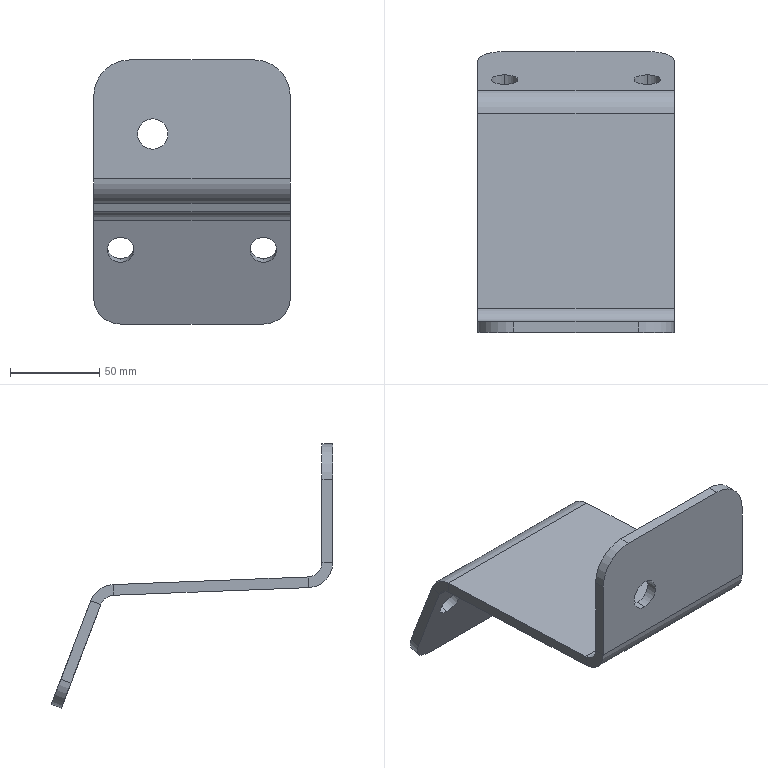Part | SolidWorks | features Fillet 2, ICE 2, FlatPattern 1, SMBaseFlange 1, SheetMetal 1 | 1 solid | 32 faces | box 110 x 157.607 x 148 mm | volume 171596 mm3 | plane 18 | cylinder 14 | commonest cylinder face diameters 15 x4 16 x2 17 x2 28 x2 30 x2 40 x2
STEP:
#1=CARTESIAN_POINT('',(-40.,133.488,-99.407));
#2=VERTEX_POINT('',#1);
#3=CARTESIAN_POINT('',(-40.,138.828,-113.424));
#4=VERTEX_POINT('',#3);
#5=CARTESIAN_POINT('',(-40.,136.158,-106.415));
#6=DIRECTION('',(0.,-0.9345,-0.356));
#7=DIRECTION('',(0.,-0.356,0.9345));
#8=AXIS2_PLACEMENT_3D('',#5,#6,#7);
#9=CIRCLE('',#8,7.5);
#10=EDGE_CURVE('',#2,#4,#9,.T.);
#11=ORIENTED_EDGE('',*,*,#10,.T.);
#12=CARTESIAN_POINT('',(-40.,144.435,-111.288));
#13=VERTEX_POINT('',#12);
#14=CARTESIAN_POINT('',(-40.,6.09,-163.991));
#15=DIRECTION('',(0.,0.9345,0.356));
#16=VECTOR('',#15,1000.);
#17=LINE('',#14,#16);
#18=EDGE_CURVE('',#4,#13,#17,.T.);
#19=ORIENTED_EDGE('',*,*,#18,.T.);
#20=CARTESIAN_POINT('',(-40.,139.095,-97.271));
#21=VERTEX_POINT('',#20);
#22=CARTESIAN_POINT('',(-40.,141.765,-104.279));
#23=DIRECTION('',(0.,0.9345,0.356));
#24=DIRECTION('',(0.,-0.356,0.9345));
#25=AXIS2_PLACEMENT_3D('',#22,#23,#24);
#26=CIRCLE('',#25,7.5);
#27=EDGE_CURVE('',#13,#21,#26,.T.);
#28=ORIENTED_EDGE('',*,*,#27,.T.);
#29=CARTESIAN_POINT('',(-40.,0.7504,-149.973));
#30=DIRECTION('',(0.,0.9345,0.356));
#31=VECTOR('',#30,1000.);
#32=LINE('',#29,#31);
#33=EDGE_CURVE('',#2,#21,#32,.T.);
#34=ORIENTED_EDGE('',*,*,#33,.F.);
#35=EDGE_LOOP('',(#11,#19,#28,#34));
#36=FACE_OUTER_BOUND('',#35,.T.);
#37=CARTESIAN_POINT('',(-40.,3.42,-156.982));
#38=DIRECTION('',(0.,0.9345,0.356));
#39=DIRECTION('',(0.,-0.356,0.9345));
#40=AXIS2_PLACEMENT_3D('',#37,#38,#39);
#41=CYLINDRICAL_SURFACE('',#40,7.5);
#42=ADVANCED_FACE('',(#36),#41,.F.);
#43=CARTESIAN_POINT('',(40.,133.488,-99.407));
#44=VERTEX_POINT('',#43);
#45=CARTESIAN_POINT('',(40.,138.828,-113.424));
#46=VERTEX_POINT('',#45);
#47=CARTESIAN_POINT('',(40.,136.158,-106.415));
#48=DIRECTION('',(0.,-0.9345,-0.356));
#49=DIRECTION('',(0.,-0.356,0.9345));
#50=AXIS2_PLACEMENT_3D('',#47,#48,#49);
#51=CIRCLE('',#50,7.5);
#52=EDGE_CURVE('',#44,#46,#51,.T.);
#53=ORIENTED_EDGE('',*,*,#52,.T.);
#54=CARTESIAN_POINT('',(40.,144.435,-111.288));
#55=VERTEX_POINT('',#54);
#56=CARTESIAN_POINT('',(40.,6.09,-163.991));
#57=DIRECTION('',(0.,0.9345,0.356));
#58=VECTOR('',#57,1000.);
#59=LINE('',#56,#58);
#60=EDGE_CURVE('',#46,#55,#59,.T.);
#61=ORIENTED_EDGE('',*,*,#60,.T.);
#62=CARTESIAN_POINT('',(40.,139.095,-97.271));
#63=VERTEX_POINT('',#62);
#64=CARTESIAN_POINT('',(40.,141.765,-104.279));
#65=DIRECTION('',(0.,0.9345,0.356));
#66=DIRECTION('',(0.,-0.356,0.9345));
#67=AXIS2_PLACEMENT_3D('',#64,#65,#66);
#68=CIRCLE('',#67,7.5);
#69=EDGE_CURVE('',#55,#63,#68,.T.);
#70=ORIENTED_EDGE('',*,*,#69,.T.);
#71=CARTESIAN_POINT('',(40.,0.7504,-149.973));
#72=DIRECTION('',(0.,0.9345,0.356));
#73=VECTOR('',#72,1000.);
#74=LINE('',#71,#73);
#75=EDGE_CURVE('',#44,#63,#74,.T.);
#76=ORIENTED_EDGE('',*,*,#75,.F.);
#77=EDGE_LOOP('',(#53,#61,#70,#76));
#78=FACE_OUTER_BOUND('',#77,.T.);
#79=CARTESIAN_POINT('',(40.,3.42,-156.982));
#80=DIRECTION('',(0.,0.9345,0.356));
#81=DIRECTION('',(0.,-0.356,0.9345));
#82=AXIS2_PLACEMENT_3D('',#79,#80,#81);
#83=CYLINDRICAL_SURFACE('',#82,7.5);
#84=ADVANCED_FACE('',(#78),#83,.F.);
#85=CARTESIAN_POINT('',(-22.,0.,-33.));
#86=VERTEX_POINT('',#85);
#87=CARTESIAN_POINT('',(-22.,0.,-50.));
#88=VERTEX_POINT('',#87);
#89=CARTESIAN_POINT('',(-22.,0.,-41.5));
#90=DIRECTION('',(0.,-1.,0.));
#91=DIRECTION('',(0.,0.,1.));
#92=AXIS2_PLACEMENT_3D('',#89,#90,#91);
#93=CIRCLE('',#92,8.5);
#94=EDGE_CURVE('',#86,#88,#93,.T.);
#95=ORIENTED_EDGE('',*,*,#94,.T.);
#96=CARTESIAN_POINT('',(-22.,6.,-50.));
#97=VERTEX_POINT('',#96);
#98=CARTESIAN_POINT('',(-22.,-0.001,-50.));
#99=DIRECTION('',(0.,1.,0.));
#100=VECTOR('',#99,1000.);
#101=LINE('',#98,#100);
#102=EDGE_CURVE('',#88,#97,#101,.T.);
#103=ORIENTED_EDGE('',*,*,#102,.T.);
#104=CARTESIAN_POINT('',(-22.,6.,-33.));
#105=VERTEX_POINT('',#104);
#106=CARTESIAN_POINT('',(-22.,6.,-41.5));
#107=DIRECTION('',(0.,1.,0.));
#108=DIRECTION('',(0.,0.,1.));
#109=AXIS2_PLACEMENT_3D('',#106,#107,#108);
#110=CIRCLE('',#109,8.5);
#111=EDGE_CURVE('',#97,#105,#110,.T.);
#112=ORIENTED_EDGE('',*,*,#111,.T.);
#113=CARTESIAN_POINT('',(-22.,-0.001,-33.));
#114=DIRECTION('',(0.,1.,0.));
#115=VECTOR('',#114,1000.);
#116=LINE('',#113,#115);
#117=EDGE_CURVE('',#86,#105,#116,.T.);
#118=ORIENTED_EDGE('',*,*,#117,.F.);
#119=EDGE_LOOP('',(#95,#103,#112,#118));
#120=FACE_OUTER_BOUND('',#119,.T.);
#121=CARTESIAN_POINT('',(-22.,-0.001,-41.5));
#122=DIRECTION('',(0.,1.,0.));
#123=DIRECTION('',(0.,0.,1.));
#124=AXIS2_PLACEMENT_3D('',#121,#122,#123);
#125=CYLINDRICAL_SURFACE('',#124,8.5);
#126=ADVANCED_FACE('',(#120),#125,.F.);
#127=CARTESIAN_POINT('',(55.,0.,-66.536));
#128=VERTEX_POINT('',#127);
#129=CARTESIAN_POINT('',(55.,6.,-66.536));
#130=VERTEX_POINT('',#129);
#131=CARTESIAN_POINT('',(55.,0.,-66.536));
#132=DIRECTION('',(0.,1.,0.));
#133=VECTOR('',#132,1000.);
#134=LINE('',#131,#133);
#135=EDGE_CURVE('',#128,#130,#134,.T.);
#136=ORIENTED_EDGE('',*,*,#135,.F.);
#137=CARTESIAN_POINT('',(55.,13.454,-80.526));
#138=VERTEX_POINT('',#137);
#139=CARTESIAN_POINT('',(55.,14.,-66.536));
#140=DIRECTION('',(1.,0.,0.));
#141=DIRECTION('',(0.,0.,1.));
#142=AXIS2_PLACEMENT_3D('',#139,#140,#141);
#143=CIRCLE('',#142,14.);
#144=EDGE_CURVE('',#128,#138,#143,.T.);
#145=ORIENTED_EDGE('',*,*,#144,.T.);
#146=CARTESIAN_POINT('',(55.,13.688,-74.53));
#147=VERTEX_POINT('',#146);
#148=CARTESIAN_POINT('',(55.,13.688,-74.53));
#149=DIRECTION('',(0.,-0.03903,-0.9992));
#150=VECTOR('',#149,1000.);
#151=LINE('',#148,#150);
#152=EDGE_CURVE('',#147,#138,#151,.T.);
#153=ORIENTED_EDGE('',*,*,#152,.F.);
#154=CARTESIAN_POINT('',(55.,14.,-66.536));
#155=DIRECTION('',(1.,0.,0.));
#156=DIRECTION('',(0.,0.,-1.));
#157=AXIS2_PLACEMENT_3D('',#154,#155,#156);
#158=CIRCLE('',#157,8.);
#159=EDGE_CURVE('',#130,#147,#158,.T.);
#160=ORIENTED_EDGE('',*,*,#159,.F.);
#161=EDGE_LOOP('',(#136,#145,#153,#160));
#162=FACE_OUTER_BOUND('',#161,.T.);
#163=CARTESIAN_POINT('',(55.,0.,-66.536));
#164=DIRECTION('',(1.,0.,0.));
#165=DIRECTION('',(0.,0.,-1.));
#166=AXIS2_PLACEMENT_3D('',#163,#164,#165);
#167=PLANE('',#166);
#168=ADVANCED_FACE('',(#162),#167,.T.);
#169=CARTESIAN_POINT('',(55.,6.,-20.));
#170=VERTEX_POINT('',#169);
#171=CARTESIAN_POINT('',(55.,6.,0.));
#172=DIRECTION('',(0.,0.,-1.));
#173=VECTOR('',#172,1000.);
#174=LINE('',#171,#173);
#175=EDGE_CURVE('',#170,#130,#174,.T.);
#176=ORIENTED_EDGE('',*,*,#175,.F.);
#177=CARTESIAN_POINT('',(55.,0.,-20.));
#178=VERTEX_POINT('',#177);
#179=CARTESIAN_POINT('',(55.,13.688,-20.));
#180=DIRECTION('',(0.,-1.,0.));
#181=VECTOR('',#180,1000.);
#182=LINE('',#179,#181);
#183=EDGE_CURVE('',#170,#178,#182,.T.);
#184=ORIENTED_EDGE('',*,*,#183,.T.);
#185=CARTESIAN_POINT('',(55.,0.,0.));
#186=DIRECTION('',(0.,0.,-1.));
#187=VECTOR('',#186,1000.);
#188=LINE('',#185,#187);
#189=EDGE_CURVE('',#178,#128,#188,.T.);
#190=ORIENTED_EDGE('',*,*,#189,.T.);
#191=ORIENTED_EDGE('',*,*,#135,.T.);
#192=EDGE_LOOP('',(#176,#184,#190,#191));
#193=FACE_OUTER_BOUND('',#192,.T.);
#194=CARTESIAN_POINT('',(55.,13.688,-74.53));
#195=DIRECTION('',(1.,0.,0.));
#196=DIRECTION('',(0.,0.,-1.));
#197=AXIS2_PLACEMENT_3D('',#194,#195,#196);
#198=PLANE('',#197);
#199=ADVANCED_FACE('',(#193),#198,.T.);
#200=CARTESIAN_POINT('',(-55.,13.454,-80.526));
#201=VERTEX_POINT('',#200);
#202=CARTESIAN_POINT('',(-55.,13.688,-74.53));
#203=VERTEX_POINT('',#202);
#204=CARTESIAN_POINT('',(-55.,13.454,-80.526));
#205=DIRECTION('',(0.,0.03903,0.9992));
#206=VECTOR('',#205,1000.);
#207=LINE('',#204,#206);
#208=EDGE_CURVE('',#201,#203,#207,.T.);
#209=ORIENTED_EDGE('',*,*,#208,.F.);
#210=CARTESIAN_POINT('',(-55.,0.,-66.536));
#211=VERTEX_POINT('',#210);
#212=CARTESIAN_POINT('',(-55.,14.,-66.536));
#213=DIRECTION('',(1.,0.,0.));
#214=DIRECTION('',(0.,0.,1.));
#215=AXIS2_PLACEMENT_3D('',#212,#213,#214);
#216=CIRCLE('',#215,14.);
#217=EDGE_CURVE('',#211,#201,#216,.T.);
#218=ORIENTED_EDGE('',*,*,#217,.F.);
#219=CARTESIAN_POINT('',(-55.,6.,-66.536));
#220=VERTEX_POINT('',#219);
#221=CARTESIAN_POINT('',(-55.,6.,-66.536));
#222=DIRECTION('',(0.,-1.,0.));
#223=VECTOR('',#222,1000.);
#224=LINE('',#221,#223);
#225=EDGE_CURVE('',#220,#211,#224,.T.);
#226=ORIENTED_EDGE('',*,*,#225,.F.);
#227=CARTESIAN_POINT('',(-55.,14.,-66.536));
#228=DIRECTION('',(1.,0.,0.));
#229=DIRECTION('',(0.,0.,-1.));
#230=AXIS2_PLACEMENT_3D('',#227,#228,#229);
#231=CIRCLE('',#230,8.);
#232=EDGE_CURVE('',#220,#203,#231,.T.);
#233=ORIENTED_EDGE('',*,*,#232,.T.);
#234=EDGE_LOOP('',(#209,#218,#226,#233));
#235=FACE_OUTER_BOUND('',#234,.T.);
#236=CARTESIAN_POINT('',(-55.,13.454,-80.526));
#237=DIRECTION('',(-1.,0.,0.));
#238=DIRECTION('',(0.,0.,1.));
#239=AXIS2_PLACEMENT_3D('',#236,#237,#238);
#240=PLANE('',#239);
#241=ADVANCED_FACE('',(#235),#240,.T.);
#242=CARTESIAN_POINT('',(-55.,122.718,-84.794));
#243=VERTEX_POINT('',#242);
#244=CARTESIAN_POINT('',(-55.,0.,-80.));
#245=DIRECTION('',(0.,0.9992,-0.03903));
#246=VECTOR('',#245,1000.);
#247=LINE('',#244,#246);
#248=EDGE_CURVE('',#201,#243,#247,.T.);
#249=ORIENTED_EDGE('',*,*,#248,.F.);
#250=ORIENTED_EDGE('',*,*,#208,.T.);
#251=CARTESIAN_POINT('',(-55.,122.952,-78.798));
#252=VERTEX_POINT('',#251);
#253=CARTESIAN_POINT('',(-55.,0.2342,-74.005));
#254=DIRECTION('',(0.,0.9992,-0.03903));
#255=VECTOR('',#254,1000.);
#256=LINE('',#253,#255);
#257=EDGE_CURVE('',#203,#252,#256,.T.);
#258=ORIENTED_EDGE('',*,*,#257,.T.);
#259=CARTESIAN_POINT('',(-55.,122.952,-78.798));
#260=DIRECTION('',(0.,-0.03903,-0.9992));
#261=VECTOR('',#260,1000.);
#262=LINE('',#259,#261);
#263=EDGE_CURVE('',#252,#243,#262,.T.);
#264=ORIENTED_EDGE('',*,*,#263,.T.);
#265=EDGE_LOOP('',(#249,#250,#258,#264));
#266=FACE_OUTER_BOUND('',#265,.T.);
#267=CARTESIAN_POINT('',(-55.,6.,-66.536));
#268=DIRECTION('',(-1.,0.,0.));
#269=DIRECTION('',(0.,0.,1.));
#270=AXIS2_PLACEMENT_3D('',#267,#268,#269);
#271=PLANE('',#270);
#272=ADVANCED_FACE('',(#266),#271,.T.);
#273=CARTESIAN_POINT('',(55.,122.718,-84.794));
#274=VERTEX_POINT('',#273);
#275=CARTESIAN_POINT('',(55.,122.952,-78.798));
#276=VERTEX_POINT('',#275);
#277=CARTESIAN_POINT('',(55.,122.718,-84.794));
#278=DIRECTION('',(0.,0.03903,0.9992));
#279=VECTOR('',#278,1000.);
#280=LINE('',#277,#279);
#281=EDGE_CURVE('',#274,#276,#280,.T.);
#282=ORIENTED_EDGE('',*,*,#281,.F.);
#283=CARTESIAN_POINT('',(55.,129.882,-89.94));
#284=VERTEX_POINT('',#283);
#285=CARTESIAN_POINT('',(55.,122.406,-92.788));
#286=DIRECTION('',(-1.,0.,0.));
#287=DIRECTION('',(0.,0.,-1.));
#288=AXIS2_PLACEMENT_3D('',#285,#286,#287);
#289=CIRCLE('',#288,8.);
#290=EDGE_CURVE('',#274,#284,#289,.T.);
#291=ORIENTED_EDGE('',*,*,#290,.T.);
#292=CARTESIAN_POINT('',(55.,135.489,-87.804));
#293=VERTEX_POINT('',#292);
#294=CARTESIAN_POINT('',(55.,135.489,-87.804));
#295=DIRECTION('',(0.,-0.9345,-0.356));
#296=VECTOR('',#295,1000.);
#297=LINE('',#294,#296);
#298=EDGE_CURVE('',#293,#284,#297,.T.);
#299=ORIENTED_EDGE('',*,*,#298,.F.);
#300=CARTESIAN_POINT('',(55.,122.406,-92.788));
#301=DIRECTION('',(-1.,0.,0.));
#302=DIRECTION('',(0.,0.,-1.));
#303=AXIS2_PLACEMENT_3D('',#300,#301,#302);
#304=CIRCLE('',#303,14.);
#305=EDGE_CURVE('',#276,#293,#304,.T.);
#306=ORIENTED_EDGE('',*,*,#305,.F.);
#307=EDGE_LOOP('',(#282,#291,#299,#306));
#308=FACE_OUTER_BOUND('',#307,.T.);
#309=CARTESIAN_POINT('',(55.,122.718,-84.794));
#310=DIRECTION('',(1.,0.,0.));
#311=DIRECTION('',(0.,0.,-1.));
#312=AXIS2_PLACEMENT_3D('',#309,#310,#311);
#313=PLANE('',#312);
#314=ADVANCED_FACE('',(#308),#313,.T.);
#315=CARTESIAN_POINT('',(55.,0.,-80.));
#316=DIRECTION('',(0.,0.9992,-0.03903));
#317=VECTOR('',#316,1000.);
#318=LINE('',#315,#317);
#319=EDGE_CURVE('',#138,#274,#318,.T.);
#320=ORIENTED_EDGE('',*,*,#319,.T.);
#321=ORIENTED_EDGE('',*,*,#281,.T.);
#322=CARTESIAN_POINT('',(55.,0.2342,-74.005));
#323=DIRECTION('',(0.,0.9992,-0.03903));
#324=VECTOR('',#323,1000.);
#325=LINE('',#322,#324);
#326=EDGE_CURVE('',#147,#276,#325,.T.);
#327=ORIENTED_EDGE('',*,*,#326,.F.);
#328=ORIENTED_EDGE('',*,*,#152,.T.);
#329=EDGE_LOOP('',(#320,#321,#327,#328));
#330=FACE_OUTER_BOUND('',#329,.T.);
#331=CARTESIAN_POINT('',(55.,135.489,-87.804));
#332=DIRECTION('',(1.,0.,0.));
#333=DIRECTION('',(0.,0.,-1.));
#334=AXIS2_PLACEMENT_3D('',#331,#332,#333);
#335=PLANE('',#334);
#336=ADVANCED_FACE('',(#330),#335,.T.);
#337=CARTESIAN_POINT('',(-55.,129.882,-89.94));
#338=VERTEX_POINT('',#337);
#339=CARTESIAN_POINT('',(-55.,135.489,-87.804));
#340=VERTEX_POINT('',#339);
#341=CARTESIAN_POINT('',(-55.,129.882,-89.94));
#342=DIRECTION('',(0.,0.9345,0.356));
#343=VECTOR('',#342,1000.);
#344=LINE('',#341,#343);
#345=EDGE_CURVE('',#338,#340,#344,.T.);
#346=ORIENTED_EDGE('',*,*,#345,.F.);
#347=CARTESIAN_POINT('',(-55.,122.406,-92.788));
#348=DIRECTION('',(-1.,0.,0.));
#349=DIRECTION('',(0.,0.,-1.));
#350=AXIS2_PLACEMENT_3D('',#347,#348,#349);
#351=CIRCLE('',#350,8.);
#352=EDGE_CURVE('',#243,#338,#351,.T.);
#353=ORIENTED_EDGE('',*,*,#352,.F.);
#354=ORIENTED_EDGE('',*,*,#263,.F.);
#355=CARTESIAN_POINT('',(-55.,122.406,-92.788));
#356=DIRECTION('',(-1.,0.,0.));
#357=DIRECTION('',(0.,0.,-1.));
#358=AXIS2_PLACEMENT_3D('',#355,#356,#357);
#359=CIRCLE('',#358,14.);
#360=EDGE_CURVE('',#252,#340,#359,.T.);
#361=ORIENTED_EDGE('',*,*,#360,.T.);
#362=EDGE_LOOP('',(#346,#353,#354,#361));
#363=FACE_OUTER_BOUND('',#362,.T.);
#364=CARTESIAN_POINT('',(-55.,129.882,-89.94));
#365=DIRECTION('',(-1.,0.,0.));
#366=DIRECTION('',(0.,0.,1.));
#367=AXIS2_PLACEMENT_3D('',#364,#365,#366);
#368=PLANE('',#367);
#369=ADVANCED_FACE('',(#363),#368,.T.);
#370=CARTESIAN_POINT('',(-55.,152.267,-131.847));
#371=VERTEX_POINT('',#370);
#372=CARTESIAN_POINT('',(-55.,133.607,-82.864));
#373=DIRECTION('',(0.,0.356,-0.9345));
#374=VECTOR('',#373,1000.);
#375=LINE('',#372,#374);
#376=EDGE_CURVE('',#340,#371,#375,.T.);
#377=ORIENTED_EDGE('',*,*,#376,.T.);
#378=CARTESIAN_POINT('',(-55.,146.66,-133.983));
#379=VERTEX_POINT('',#378);
#380=CARTESIAN_POINT('',(-55.,144.315,-134.876));
#381=DIRECTION('',(0.,-0.9345,-0.356));
#382=VECTOR('',#381,1000.);
#383=LINE('',#380,#382);
#384=EDGE_CURVE('',#371,#379,#383,.T.);
#385=ORIENTED_EDGE('',*,*,#384,.T.);
#386=CARTESIAN_POINT('',(-55.,128.,-85.));
#387=DIRECTION('',(0.,0.356,-0.9345));
#388=VECTOR('',#387,1000.);
#389=LINE('',#386,#388);
#390=EDGE_CURVE('',#338,#379,#389,.T.);
#391=ORIENTED_EDGE('',*,*,#390,.F.);
#392=ORIENTED_EDGE('',*,*,#345,.T.);
#393=EDGE_LOOP('',(#377,#385,#391,#392));
#394=FACE_OUTER_BOUND('',#393,.T.);
#395=CARTESIAN_POINT('',(-55.,122.952,-78.798));
#396=DIRECTION('',(-1.,0.,0.));
#397=DIRECTION('',(0.,0.,1.));
#398=AXIS2_PLACEMENT_3D('',#395,#396,#397);
#399=PLANE('',#398);
#400=ADVANCED_FACE('',(#394),#399,.T.);
#401=ORIENTED_EDGE('',*,*,#10,.F.);
#402=CARTESIAN_POINT('',(-40.,136.158,-106.415));
#403=DIRECTION('',(0.,-0.9345,-0.356));
#404=DIRECTION('',(0.,-0.356,0.9345));
#405=AXIS2_PLACEMENT_3D('',#402,#403,#404);
#406=CIRCLE('',#405,7.5);
#407=EDGE_CURVE('',#4,#2,#406,.T.);
#408=ORIENTED_EDGE('',*,*,#407,.F.);
#409=EDGE_LOOP('',(#401,#408));
#410=FACE_BOUND('',#409,.T.);
#411=ORIENTED_EDGE('',*,*,#52,.F.);
#412=CARTESIAN_POINT('',(40.,136.158,-106.415));
#413=DIRECTION('',(0.,-0.9345,-0.356));
#414=DIRECTION('',(0.,-0.356,0.9345));
#415=AXIS2_PLACEMENT_3D('',#412,#413,#414);
#416=CIRCLE('',#415,7.5);
#417=EDGE_CURVE('',#46,#44,#416,.T.);
#418=ORIENTED_EDGE('',*,*,#417,.F.);
#419=EDGE_LOOP('',(#411,#418));
#420=FACE_BOUND('',#419,.T.);
#421=ORIENTED_EDGE('',*,*,#390,.T.);
#422=CARTESIAN_POINT('',(-40.,152.,-148.));
#423=VERTEX_POINT('',#422);
#424=CARTESIAN_POINT('',(-40.,146.66,-133.983));
#425=DIRECTION('',(0.,-0.9345,-0.356));
#426=DIRECTION('',(0.,-0.356,0.9345));
#427=AXIS2_PLACEMENT_3D('',#424,#425,#426);
#428=CIRCLE('',#427,15.);
#429=EDGE_CURVE('',#379,#423,#428,.T.);
#430=ORIENTED_EDGE('',*,*,#429,.T.);
#431=CARTESIAN_POINT('',(40.,152.,-148.));
#432=VERTEX_POINT('',#431);
#433=CARTESIAN_POINT('',(55.,152.,-148.));
#434=DIRECTION('',(-1.,0.,0.));
#435=VECTOR('',#434,1000.);
#436=LINE('',#433,#435);
#437=EDGE_CURVE('',#432,#423,#436,.T.);
#438=ORIENTED_EDGE('',*,*,#437,.F.);
#439=CARTESIAN_POINT('',(55.,146.66,-133.983));
#440=VERTEX_POINT('',#439);
#441=CARTESIAN_POINT('',(40.,146.66,-133.983));
#442=DIRECTION('',(0.,-0.9345,-0.356));
#443=DIRECTION('',(0.,-0.356,0.9345));
#444=AXIS2_PLACEMENT_3D('',#441,#442,#443);
#445=CIRCLE('',#444,15.);
#446=EDGE_CURVE('',#432,#440,#445,.T.);
#447=ORIENTED_EDGE('',*,*,#446,.T.);
#448=CARTESIAN_POINT('',(55.,128.,-85.));
#449=DIRECTION('',(0.,0.356,-0.9345));
#450=VECTOR('',#449,1000.);
#451=LINE('',#448,#450);
#452=EDGE_CURVE('',#284,#440,#451,.T.);
#453=ORIENTED_EDGE('',*,*,#452,.F.);
#454=CARTESIAN_POINT('',(55.,129.882,-89.94));
#455=DIRECTION('',(-1.,0.,0.));
#456=VECTOR('',#455,1000.);
#457=LINE('',#454,#456);
#458=EDGE_CURVE('',#284,#338,#457,.T.);
#459=ORIENTED_EDGE('',*,*,#458,.T.);
#460=EDGE_LOOP('',(#421,#430,#438,#447,#453,#459));
#461=FACE_OUTER_BOUND('',#460,.T.);
#462=CARTESIAN_POINT('',(55.,128.,-85.));
#463=DIRECTION('',(0.,0.9345,0.356));
#464=DIRECTION('',(0.,-0.356,0.9345));
#465=AXIS2_PLACEMENT_3D('',#462,#463,#464);
#466=PLANE('',#465);
#467=ADVANCED_FACE('',(#410,#420,#461),#466,.F.);
#468=ORIENTED_EDGE('',*,*,#437,.T.);
#469=CARTESIAN_POINT('',(-40.,157.607,-145.864));
#470=VERTEX_POINT('',#469);
#471=CARTESIAN_POINT('',(-40.,157.607,-145.864));
#472=DIRECTION('',(0.,0.9345,0.356));
#473=VECTOR('',#472,1000.);
#474=LINE('',#471,#473);
#475=EDGE_CURVE('',#423,#470,#474,.T.);
#476=ORIENTED_EDGE('',*,*,#475,.T.);
#477=CARTESIAN_POINT('',(40.,157.607,-145.864));
#478=VERTEX_POINT('',#477);
#479=CARTESIAN_POINT('',(55.,157.607,-145.864));
#480=DIRECTION('',(-1.,0.,0.));
#481=VECTOR('',#480,1000.);
#482=LINE('',#479,#481);
#483=EDGE_CURVE('',#478,#470,#482,.T.);
#484=ORIENTED_EDGE('',*,*,#483,.F.);
#485=CARTESIAN_POINT('',(40.,157.607,-145.864));
#486=DIRECTION('',(0.,-0.9345,-0.356));
#487=VECTOR('',#486,1000.);
#488=LINE('',#485,#487);
#489=EDGE_CURVE('',#478,#432,#488,.T.);
#490=ORIENTED_EDGE('',*,*,#489,.T.);
#491=EDGE_LOOP('',(#468,#476,#484,#490));
#492=FACE_OUTER_BOUND('',#491,.T.);
#493=CARTESIAN_POINT('',(55.,157.607,-145.864));
#494=DIRECTION('',(0.,0.356,-0.9345));
#495=DIRECTION('',(0.,0.9345,0.356));
#496=AXIS2_PLACEMENT_3D('',#493,#494,#495);
#497=PLANE('',#496);
#498=ADVANCED_FACE('',(#492),#497,.T.);
#499=CARTESIAN_POINT('',(-40.,141.765,-104.279));
#500=DIRECTION('',(0.,0.9345,0.356));
#501=DIRECTION('',(0.,-0.356,0.9345));
#502=AXIS2_PLACEMENT_3D('',#499,#500,#501);
#503=CIRCLE('',#502,7.5);
#504=EDGE_CURVE('',#21,#13,#503,.T.);
#505=ORIENTED_EDGE('',*,*,#504,.F.);
#506=ORIENTED_EDGE('',*,*,#27,.F.);
#507=EDGE_LOOP('',(#505,#506));
#508=FACE_BOUND('',#507,.T.);
#509=CARTESIAN_POINT('',(40.,141.765,-104.279));
#510=DIRECTION('',(0.,0.9345,0.356));
#511=DIRECTION('',(0.,-0.356,0.9345));
#512=AXIS2_PLACEMENT_3D('',#509,#510,#511);
#513=CIRCLE('',#512,7.5);
#514=EDGE_CURVE('',#63,#55,#513,.T.);
#515=ORIENTED_EDGE('',*,*,#514,.F.);
#516=ORIENTED_EDGE('',*,*,#69,.F.);
#517=EDGE_LOOP('',(#515,#516));
#518=FACE_BOUND('',#517,.T.);
#519=ORIENTED_EDGE('',*,*,#483,.T.);
#520=CARTESIAN_POINT('',(-40.,152.267,-131.847));
#521=DIRECTION('',(0.,0.9345,0.356));
#522=DIRECTION('',(0.,-0.356,0.9345));
#523=AXIS2_PLACEMENT_3D('',#520,#521,#522);
#524=CIRCLE('',#523,15.);
#525=EDGE_CURVE('',#470,#371,#524,.T.);
#526=ORIENTED_EDGE('',*,*,#525,.T.);
#527=ORIENTED_EDGE('',*,*,#376,.F.);
#528=CARTESIAN_POINT('',(55.,135.489,-87.804));
#529=DIRECTION('',(-1.,0.,0.));
#530=VECTOR('',#529,1000.);
#531=LINE('',#528,#530);
#532=EDGE_CURVE('',#293,#340,#531,.T.);
#533=ORIENTED_EDGE('',*,*,#532,.F.);
#534=CARTESIAN_POINT('',(55.,152.267,-131.847));
#535=VERTEX_POINT('',#534);
#536=CARTESIAN_POINT('',(55.,133.607,-82.864));
#537=DIRECTION('',(0.,0.356,-0.9345));
#538=VECTOR('',#537,1000.);
#539=LINE('',#536,#538);
#540=EDGE_CURVE('',#293,#535,#539,.T.);
#541=ORIENTED_EDGE('',*,*,#540,.T.);
#542=CARTESIAN_POINT('',(40.,152.267,-131.847));
#543=DIRECTION('',(0.,0.9345,0.356));
#544=DIRECTION('',(0.,-0.356,0.9345));
#545=AXIS2_PLACEMENT_3D('',#542,#543,#544);
#546=CIRCLE('',#545,15.);
#547=EDGE_CURVE('',#535,#478,#546,.T.);
#548=ORIENTED_EDGE('',*,*,#547,.T.);
#549=EDGE_LOOP('',(#519,#526,#527,#533,#541,#548));
#550=FACE_OUTER_BOUND('',#549,.T.);
#551=CARTESIAN_POINT('',(55.,133.607,-82.864));
#552=DIRECTION('',(0.,0.9345,0.356));
#553=DIRECTION('',(0.,-0.356,0.9345));
#554=AXIS2_PLACEMENT_3D('',#551,#552,#553);
#555=PLANE('',#554);
#556=ADVANCED_FACE('',(#508,#518,#550),#555,.T.);
#557=ORIENTED_EDGE('',*,*,#360,.F.);
#558=CARTESIAN_POINT('',(55.,122.952,-78.798));
#559=DIRECTION('',(-1.,0.,0.));
#560=VECTOR('',#559,1000.);
#561=LINE('',#558,#560);
#562=EDGE_CURVE('',#276,#252,#561,.T.);
#563=ORIENTED_EDGE('',*,*,#562,.F.);
#564=ORIENTED_EDGE('',*,*,#305,.T.);
#565=ORIENTED_EDGE('',*,*,#532,.T.);
#566=EDGE_LOOP('',(#557,#563,#564,#565));
#567=FACE_OUTER_BOUND('',#566,.T.);
#568=CARTESIAN_POINT('',(55.,122.406,-92.788));
#569=DIRECTION('',(-1.,0.,0.));
#570=DIRECTION('',(0.,0.,1.));
#571=AXIS2_PLACEMENT_3D('',#568,#569,#570);
#572=CYLINDRICAL_SURFACE('',#571,14.);
#573=ADVANCED_FACE('',(#567),#572,.T.);
#574=ORIENTED_EDGE('',*,*,#257,.F.);
#575=CARTESIAN_POINT('',(55.,13.688,-74.53));
#576=DIRECTION('',(-1.,0.,0.));
#577=VECTOR('',#576,1000.);
#578=LINE('',#575,#577);
#579=EDGE_CURVE('',#147,#203,#578,.T.);
#580=ORIENTED_EDGE('',*,*,#579,.F.);
#581=ORIENTED_EDGE('',*,*,#326,.T.);
#582=ORIENTED_EDGE('',*,*,#562,.T.);
#583=EDGE_LOOP('',(#574,#580,#581,#582));
#584=FACE_OUTER_BOUND('',#583,.T.);
#585=CARTESIAN_POINT('',(55.,0.2342,-74.005));
#586=DIRECTION('',(0.,0.03903,0.9992));
#587=DIRECTION('',(0.,-0.9992,0.03903));
#588=AXIS2_PLACEMENT_3D('',#585,#586,#587);
#589=PLANE('',#588);
#590=ADVANCED_FACE('',(#584),#589,.T.);
#591=ORIENTED_EDGE('',*,*,#232,.F.);
#592=CARTESIAN_POINT('',(55.,6.,-66.536));
#593=DIRECTION('',(-1.,0.,0.));
#594=VECTOR('',#593,1000.);
#595=LINE('',#592,#594);
#596=EDGE_CURVE('',#130,#220,#595,.T.);
#597=ORIENTED_EDGE('',*,*,#596,.F.);
#598=ORIENTED_EDGE('',*,*,#159,.T.);
#599=ORIENTED_EDGE('',*,*,#579,.T.);
#600=EDGE_LOOP('',(#591,#597,#598,#599));
#601=FACE_OUTER_BOUND('',#600,.T.);
#602=CARTESIAN_POINT('',(55.,14.,-66.536));
#603=DIRECTION('',(-1.,0.,0.));
#604=DIRECTION('',(0.,0.,1.));
#605=AXIS2_PLACEMENT_3D('',#602,#603,#604);
#606=CYLINDRICAL_SURFACE('',#605,8.);
#607=ADVANCED_FACE('',(#601),#606,.F.);
#608=CARTESIAN_POINT('',(-22.,6.,-41.5));
#609=DIRECTION('',(0.,1.,0.));
#610=DIRECTION('',(0.,0.,1.));
#611=AXIS2_PLACEMENT_3D('',#608,#609,#610);
#612=CIRCLE('',#611,8.5);
#613=EDGE_CURVE('',#105,#97,#612,.T.);
#614=ORIENTED_EDGE('',*,*,#613,.F.);
#615=ORIENTED_EDGE('',*,*,#111,.F.);
#616=EDGE_LOOP('',(#614,#615));
#617=FACE_BOUND('',#616,.T.);
#618=CARTESIAN_POINT('',(35.,6.,0.));
#619=VERTEX_POINT('',#618);
#620=CARTESIAN_POINT('',(-35.,6.,0.));
#621=VERTEX_POINT('',#620);
#622=CARTESIAN_POINT('',(55.,6.,0.));
#623=DIRECTION('',(-1.,0.,0.));
#624=VECTOR('',#623,1000.);
#625=LINE('',#622,#624);
#626=EDGE_CURVE('',#619,#621,#625,.T.);
#627=ORIENTED_EDGE('',*,*,#626,.F.);
#628=CARTESIAN_POINT('',(35.,6.,-20.));
#629=DIRECTION('',(0.,1.,0.));
#630=DIRECTION('',(0.,0.,1.));
#631=AXIS2_PLACEMENT_3D('',#628,#629,#630);
#632=CIRCLE('',#631,20.);
#633=EDGE_CURVE('',#619,#170,#632,.T.);
#634=ORIENTED_EDGE('',*,*,#633,.T.);
#635=ORIENTED_EDGE('',*,*,#175,.T.);
#636=ORIENTED_EDGE('',*,*,#596,.T.);
#637=CARTESIAN_POINT('',(-55.,6.,-20.));
#638=VERTEX_POINT('',#637);
#639=CARTESIAN_POINT('',(-55.,6.,0.));
#640=DIRECTION('',(0.,0.,-1.));
#641=VECTOR('',#640,1000.);
#642=LINE('',#639,#641);
#643=EDGE_CURVE('',#638,#220,#642,.T.);
#644=ORIENTED_EDGE('',*,*,#643,.F.);
#645=CARTESIAN_POINT('',(-35.,6.,-20.));
#646=DIRECTION('',(0.,1.,0.));
#647=DIRECTION('',(0.,0.,1.));
#648=AXIS2_PLACEMENT_3D('',#645,#646,#647);
#649=CIRCLE('',#648,20.);
#650=EDGE_CURVE('',#638,#621,#649,.T.);
#651=ORIENTED_EDGE('',*,*,#650,.T.);
#652=EDGE_LOOP('',(#627,#634,#635,#636,#644,#651));
#653=FACE_OUTER_BOUND('',#652,.T.);
#654=CARTESIAN_POINT('',(55.,6.,0.));
#655=DIRECTION('',(0.,1.,0.));
#656=DIRECTION('',(0.,0.,1.));
#657=AXIS2_PLACEMENT_3D('',#654,#655,#656);
#658=PLANE('',#657);
#659=ADVANCED_FACE('',(#617,#653),#658,.T.);
#660=CARTESIAN_POINT('',(35.,0.,0.));
#661=VERTEX_POINT('',#660);
#662=CARTESIAN_POINT('',(-35.,0.,0.));
#663=VERTEX_POINT('',#662);
#664=CARTESIAN_POINT('',(55.,0.,0.));
#665=DIRECTION('',(-1.,0.,0.));
#666=VECTOR('',#665,1000.);
#667=LINE('',#664,#666);
#668=EDGE_CURVE('',#661,#663,#667,.T.);
#669=ORIENTED_EDGE('',*,*,#668,.F.);
#670=CARTESIAN_POINT('',(35.,0.,0.));
#671=DIRECTION('',(0.,1.,0.));
#672=VECTOR('',#671,1000.);
#673=LINE('',#670,#672);
#674=EDGE_CURVE('',#661,#619,#673,.T.);
#675=ORIENTED_EDGE('',*,*,#674,.T.);
#676=ORIENTED_EDGE('',*,*,#626,.T.);
#677=CARTESIAN_POINT('',(-35.,0.,0.));
#678=DIRECTION('',(0.,-1.,0.));
#679=VECTOR('',#678,1000.);
#680=LINE('',#677,#679);
#681=EDGE_CURVE('',#621,#663,#680,.T.);
#682=ORIENTED_EDGE('',*,*,#681,.T.);
#683=EDGE_LOOP('',(#669,#675,#676,#682));
#684=FACE_OUTER_BOUND('',#683,.T.);
#685=CARTESIAN_POINT('',(55.,0.,0.));
#686=DIRECTION('',(0.,0.,1.));
#687=DIRECTION('',(1.,0.,0.));
#688=AXIS2_PLACEMENT_3D('',#685,#686,#687);
#689=PLANE('',#688);
#690=ADVANCED_FACE('',(#684),#689,.T.);
#691=ORIENTED_EDGE('',*,*,#94,.F.);
#692=CARTESIAN_POINT('',(-22.,0.,-41.5));
#693=DIRECTION('',(0.,-1.,0.));
#694=DIRECTION('',(0.,0.,1.));
#695=AXIS2_PLACEMENT_3D('',#692,#693,#694);
#696=CIRCLE('',#695,8.5);
#697=EDGE_CURVE('',#88,#86,#696,.T.);
#698=ORIENTED_EDGE('',*,*,#697,.F.);
#699=EDGE_LOOP('',(#691,#698));
#700=FACE_BOUND('',#699,.T.);
#701=ORIENTED_EDGE('',*,*,#189,.F.);
#702=CARTESIAN_POINT('',(35.,0.,-20.));
#703=DIRECTION('',(0.,-1.,0.));
#704=DIRECTION('',(0.,0.,1.));
#705=AXIS2_PLACEMENT_3D('',#702,#703,#704);
#706=CIRCLE('',#705,20.);
#707=EDGE_CURVE('',#178,#661,#706,.T.);
#708=ORIENTED_EDGE('',*,*,#707,.T.);
#709=ORIENTED_EDGE('',*,*,#668,.T.);
#710=CARTESIAN_POINT('',(-55.,0.,-20.));
#711=VERTEX_POINT('',#710);
#712=CARTESIAN_POINT('',(-35.,0.,-20.));
#713=DIRECTION('',(0.,-1.,0.));
#714=DIRECTION('',(0.,0.,1.));
#715=AXIS2_PLACEMENT_3D('',#712,#713,#714);
#716=CIRCLE('',#715,20.);
#717=EDGE_CURVE('',#663,#711,#716,.T.);
#718=ORIENTED_EDGE('',*,*,#717,.T.);
#719=CARTESIAN_POINT('',(-55.,0.,0.));
#720=DIRECTION('',(0.,0.,-1.));
#721=VECTOR('',#720,1000.);
#722=LINE('',#719,#721);
#723=EDGE_CURVE('',#711,#211,#722,.T.);
#724=ORIENTED_EDGE('',*,*,#723,.T.);
#725=CARTESIAN_POINT('',(55.,0.,-66.536));
#726=DIRECTION('',(-1.,0.,0.));
#727=VECTOR('',#726,1000.);
#728=LINE('',#725,#727);
#729=EDGE_CURVE('',#128,#211,#728,.T.);
#730=ORIENTED_EDGE('',*,*,#729,.F.);
#731=EDGE_LOOP('',(#701,#708,#709,#718,#724,#730));
#732=FACE_OUTER_BOUND('',#731,.T.);
#733=CARTESIAN_POINT('',(55.,0.,0.));
#734=DIRECTION('',(0.,1.,0.));
#735=DIRECTION('',(0.,0.,1.));
#736=AXIS2_PLACEMENT_3D('',#733,#734,#735);
#737=PLANE('',#736);
#738=ADVANCED_FACE('',(#700,#732),#737,.F.);
#739=ORIENTED_EDGE('',*,*,#217,.T.);
#740=CARTESIAN_POINT('',(55.,13.454,-80.526));
#741=DIRECTION('',(-1.,0.,0.));
#742=VECTOR('',#741,1000.);
#743=LINE('',#740,#742);
#744=EDGE_CURVE('',#138,#201,#743,.T.);
#745=ORIENTED_EDGE('',*,*,#744,.F.);
#746=ORIENTED_EDGE('',*,*,#144,.F.);
#747=ORIENTED_EDGE('',*,*,#729,.T.);
#748=EDGE_LOOP('',(#739,#745,#746,#747));
#749=FACE_OUTER_BOUND('',#748,.T.);
#750=CARTESIAN_POINT('',(55.,14.,-66.536));
#751=DIRECTION('',(-1.,0.,0.));
#752=DIRECTION('',(0.,0.,1.));
#753=AXIS2_PLACEMENT_3D('',#750,#751,#752);
#754=CYLINDRICAL_SURFACE('',#753,14.);
#755=ADVANCED_FACE('',(#749),#754,.T.);
#756=ORIENTED_EDGE('',*,*,#248,.T.);
#757=CARTESIAN_POINT('',(55.,122.718,-84.794));
#758=DIRECTION('',(-1.,0.,0.));
#759=VECTOR('',#758,1000.);
#760=LINE('',#757,#759);
#761=EDGE_CURVE('',#274,#243,#760,.T.);
#762=ORIENTED_EDGE('',*,*,#761,.F.);
#763=ORIENTED_EDGE('',*,*,#319,.F.);
#764=ORIENTED_EDGE('',*,*,#744,.T.);
#765=EDGE_LOOP('',(#756,#762,#763,#764));
#766=FACE_OUTER_BOUND('',#765,.T.);
#767=CARTESIAN_POINT('',(55.,0.,-80.));
#768=DIRECTION('',(0.,0.03903,0.9992));
#769=DIRECTION('',(0.,-0.9992,0.03903));
#770=AXIS2_PLACEMENT_3D('',#767,#768,#769);
#771=PLANE('',#770);
#772=ADVANCED_FACE('',(#766),#771,.F.);
#773=ORIENTED_EDGE('',*,*,#352,.T.);
#774=ORIENTED_EDGE('',*,*,#458,.F.);
#775=ORIENTED_EDGE('',*,*,#290,.F.);
#776=ORIENTED_EDGE('',*,*,#761,.T.);
#777=EDGE_LOOP('',(#773,#774,#775,#776));
#778=FACE_OUTER_BOUND('',#777,.T.);
#779=CARTESIAN_POINT('',(55.,122.406,-92.788));
#780=DIRECTION('',(-1.,0.,0.));
#781=DIRECTION('',(0.,0.,1.));
#782=AXIS2_PLACEMENT_3D('',#779,#780,#781);
#783=CYLINDRICAL_SURFACE('',#782,8.);
#784=ADVANCED_FACE('',(#778),#783,.F.);
#785=ORIENTED_EDGE('',*,*,#452,.T.);
#786=CARTESIAN_POINT('',(55.,139.184,-136.831));
#787=DIRECTION('',(0.,0.9345,0.356));
#788=VECTOR('',#787,1000.);
#789=LINE('',#786,#788);
#790=EDGE_CURVE('',#440,#535,#789,.T.);
#791=ORIENTED_EDGE('',*,*,#790,.T.);
#792=ORIENTED_EDGE('',*,*,#540,.F.);
#793=ORIENTED_EDGE('',*,*,#298,.T.);
#794=EDGE_LOOP('',(#785,#791,#792,#793));
#795=FACE_OUTER_BOUND('',#794,.T.);
#796=CARTESIAN_POINT('',(55.,122.406,-92.788));
#797=DIRECTION('',(1.,0.,0.));
#798=DIRECTION('',(0.,0.,-1.));
#799=AXIS2_PLACEMENT_3D('',#796,#797,#798);
#800=PLANE('',#799);
#801=ADVANCED_FACE('',(#795),#800,.T.);
#802=ORIENTED_EDGE('',*,*,#723,.F.);
#803=CARTESIAN_POINT('',(-55.,6.,-20.));
#804=DIRECTION('',(0.,1.,0.));
#805=VECTOR('',#804,1000.);
#806=LINE('',#803,#805);
#807=EDGE_CURVE('',#711,#638,#806,.T.);
#808=ORIENTED_EDGE('',*,*,#807,.T.);
#809=ORIENTED_EDGE('',*,*,#643,.T.);
#810=ORIENTED_EDGE('',*,*,#225,.T.);
#811=EDGE_LOOP('',(#802,#808,#809,#810));
#812=FACE_OUTER_BOUND('',#811,.T.);
#813=CARTESIAN_POINT('',(-55.,122.406,-92.788));
#814=DIRECTION('',(1.,0.,0.));
#815=DIRECTION('',(0.,0.,-1.));
#816=AXIS2_PLACEMENT_3D('',#813,#814,#815);
#817=PLANE('',#816);
#818=ADVANCED_FACE('',(#812),#817,.F.);
#819=ORIENTED_EDGE('',*,*,#102,.F.);
#820=ORIENTED_EDGE('',*,*,#697,.T.);
#821=ORIENTED_EDGE('',*,*,#117,.T.);
#822=ORIENTED_EDGE('',*,*,#613,.T.);
#823=EDGE_LOOP('',(#819,#820,#821,#822));
#824=FACE_OUTER_BOUND('',#823,.T.);
#825=CARTESIAN_POINT('',(-22.,-0.001,-41.5));
#826=DIRECTION('',(0.,1.,0.));
#827=DIRECTION('',(0.,0.,1.));
#828=AXIS2_PLACEMENT_3D('',#825,#826,#827);
#829=CYLINDRICAL_SURFACE('',#828,8.5);
#830=ADVANCED_FACE('',(#824),#829,.F.);
#831=ORIENTED_EDGE('',*,*,#60,.F.);
#832=ORIENTED_EDGE('',*,*,#417,.T.);
#833=ORIENTED_EDGE('',*,*,#75,.T.);
#834=ORIENTED_EDGE('',*,*,#514,.T.);
#835=EDGE_LOOP('',(#831,#832,#833,#834));
#836=FACE_OUTER_BOUND('',#835,.T.);
#837=CARTESIAN_POINT('',(40.,3.42,-156.982));
#838=DIRECTION('',(0.,0.9345,0.356));
#839=DIRECTION('',(0.,-0.356,0.9345));
#840=AXIS2_PLACEMENT_3D('',#837,#838,#839);
#841=CYLINDRICAL_SURFACE('',#840,7.5);
#842=ADVANCED_FACE('',(#836),#841,.F.);
#843=ORIENTED_EDGE('',*,*,#18,.F.);
#844=ORIENTED_EDGE('',*,*,#407,.T.);
#845=ORIENTED_EDGE('',*,*,#33,.T.);
#846=ORIENTED_EDGE('',*,*,#504,.T.);
#847=EDGE_LOOP('',(#843,#844,#845,#846));
#848=FACE_OUTER_BOUND('',#847,.T.);
#849=CARTESIAN_POINT('',(-40.,3.42,-156.982));
#850=DIRECTION('',(0.,0.9345,0.356));
#851=DIRECTION('',(0.,-0.356,0.9345));
#852=AXIS2_PLACEMENT_3D('',#849,#850,#851);
#853=CYLINDRICAL_SURFACE('',#852,7.5);
#854=ADVANCED_FACE('',(#848),#853,.F.);
#855=ORIENTED_EDGE('',*,*,#707,.F.);
#856=ORIENTED_EDGE('',*,*,#183,.F.);
#857=ORIENTED_EDGE('',*,*,#633,.F.);
#858=ORIENTED_EDGE('',*,*,#674,.F.);
#859=EDGE_LOOP('',(#855,#856,#857,#858));
#860=FACE_OUTER_BOUND('',#859,.T.);
#861=CARTESIAN_POINT('',(35.,0.,-20.));
#862=DIRECTION('',(0.,1.,0.));
#863=DIRECTION('',(0.,0.,1.));
#864=AXIS2_PLACEMENT_3D('',#861,#862,#863);
#865=CYLINDRICAL_SURFACE('',#864,20.);
#866=ADVANCED_FACE('',(#860),#865,.T.);
#867=ORIENTED_EDGE('',*,*,#717,.F.);
#868=ORIENTED_EDGE('',*,*,#681,.F.);
#869=ORIENTED_EDGE('',*,*,#650,.F.);
#870=ORIENTED_EDGE('',*,*,#807,.F.);
#871=EDGE_LOOP('',(#867,#868,#869,#870));
#872=FACE_OUTER_BOUND('',#871,.T.);
#873=CARTESIAN_POINT('',(-35.,122.406,-20.));
#874=DIRECTION('',(0.,-1.,0.));
#875=DIRECTION('',(0.,0.,-1.));
#876=AXIS2_PLACEMENT_3D('',#873,#874,#875);
#877=CYLINDRICAL_SURFACE('',#876,20.);
#878=ADVANCED_FACE('',(#872),#877,.T.);
#879=ORIENTED_EDGE('',*,*,#525,.F.);
#880=ORIENTED_EDGE('',*,*,#475,.F.);
#881=ORIENTED_EDGE('',*,*,#429,.F.);
#882=ORIENTED_EDGE('',*,*,#384,.F.);
#883=EDGE_LOOP('',(#879,#880,#881,#882));
#884=FACE_OUTER_BOUND('',#883,.T.);
#885=CARTESIAN_POINT('',(-40.,144.315,-134.876));
#886=DIRECTION('',(0.,-0.9345,-0.356));
#887=DIRECTION('',(0.,0.356,-0.9345));
#888=AXIS2_PLACEMENT_3D('',#885,#886,#887);
#889=CYLINDRICAL_SURFACE('',#888,15.);
#890=ADVANCED_FACE('',(#884),#889,.T.);
#891=ORIENTED_EDGE('',*,*,#547,.F.);
#892=ORIENTED_EDGE('',*,*,#790,.F.);
#893=ORIENTED_EDGE('',*,*,#446,.F.);
#894=ORIENTED_EDGE('',*,*,#489,.F.);
#895=EDGE_LOOP('',(#891,#892,#893,#894));
#896=FACE_OUTER_BOUND('',#895,.T.);
#897=CARTESIAN_POINT('',(40.,152.267,-131.847));
#898=DIRECTION('',(0.,-0.9345,-0.356));
#899=DIRECTION('',(0.,0.356,-0.9345));
#900=AXIS2_PLACEMENT_3D('',#897,#898,#899);
#901=CYLINDRICAL_SURFACE('',#900,15.);
#902=ADVANCED_FACE('',(#896),#901,.T.);
#903=CLOSED_SHELL('',(#42,#84,#126,#168,#199,#241,#272,#314,#336,#369,#400,#467,#498,#556,#573,#590,#607,#659,#690,#738,#755,#772,#784,#801,#818,#830,#842,#854,#866,#878,#890,#902));
#904=MANIFOLD_SOLID_BREP('',#903);
#905=CARTESIAN_POINT('',(0.,0.,0.));
#906=DIRECTION('',(0.,0.,1.));
#907=DIRECTION('',(1.,0.,0.));
#908=AXIS2_PLACEMENT_3D('',#905,#906,#907);
#909=(LENGTH_UNIT()NAMED_UNIT(*)SI_UNIT(.MILLI.,.METRE.));
#910=UNCERTAINTY_MEASURE_WITH_UNIT(LENGTH_MEASURE(0.00001),#909,'','');
#911=(NAMED_UNIT(*)PLANE_ANGLE_UNIT()SI_UNIT($,.RADIAN.));
#912=(NAMED_UNIT(*)SI_UNIT($,.STERADIAN.)SOLID_ANGLE_UNIT());
#913=(GEOMETRIC_REPRESENTATION_CONTEXT(3)GLOBAL_UNCERTAINTY_ASSIGNED_CONTEXT((#910))GLOBAL_UNIT_ASSIGNED_CONTEXT((#909,#911,#912))REPRESENTATION_CONTEXT('',''));
#914=ADVANCED_BREP_SHAPE_REPRESENTATION('',(#904,#908),#913);